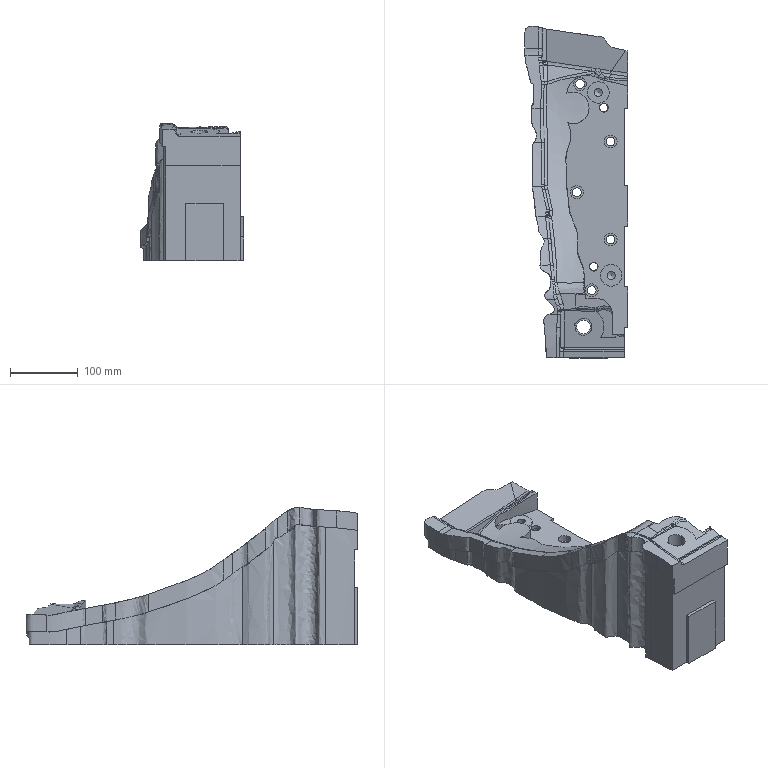Part | NX | features solid 2 | 1 solid | 247 faces | box 152.491 x 490.724 x 202.902 mm | volume 4380932 mm3 | spline 148 | plane 49 | cylinder 45 | sphere 3 | cone 2 | commonest cylinder face diameters 12 x10 13 x7 10 x6 19 x5 32 x2 4 x1